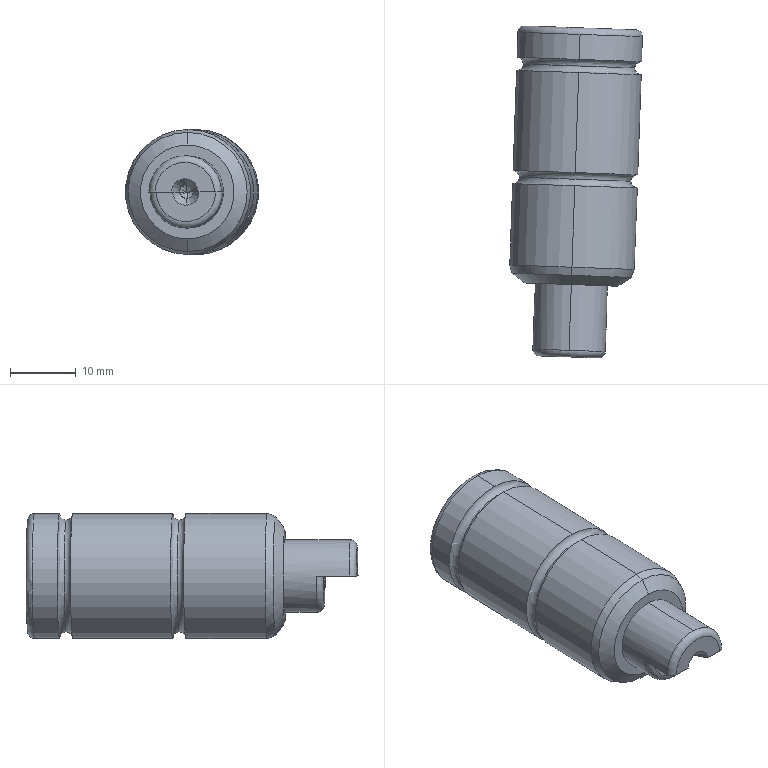Part | NX | features 1 2 | 1 solid | 173 faces | box 20.223 x 50.424 x 19 mm | volume 11414 mm3 | plane 109 | spline 31 | cylinder 14 | cone 12 | torus 7 | commonest cylinder face diameters 19 x6 2 x4 4.9 x2 11 x2